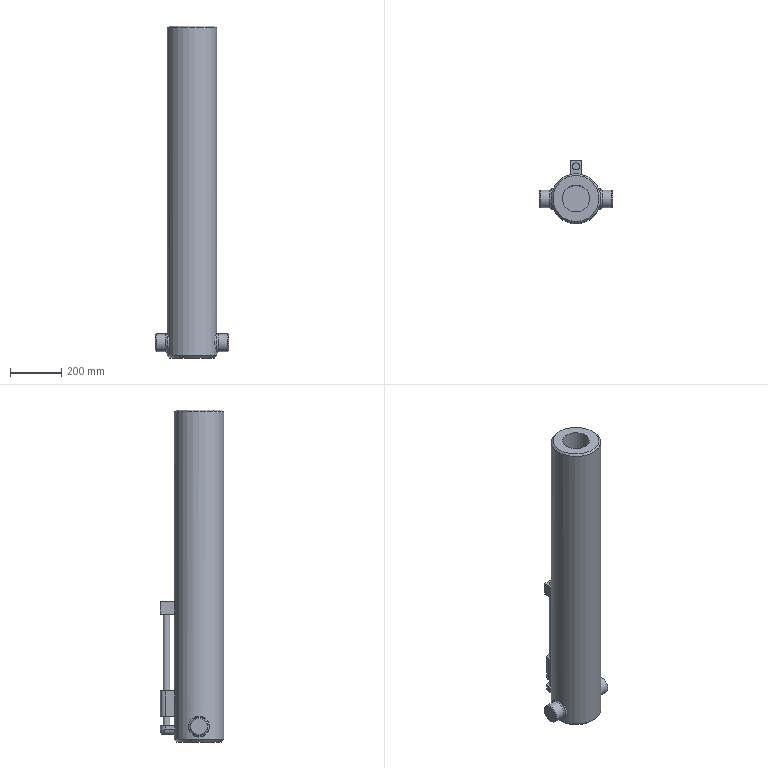Part | NX | features 推移千斤顶缸 2 | 1 solid | 49 faces | box 287 x 247.6 x 1299 mm | volume 29707096 mm3 | plane 23 | cylinder 18 | cone 4 | torus 2 | spline 2 | commonest cylinder face diameters 40 x6 81.5 x4 28.35 x2 70 x2 20 x1 28 x1
STEP:
#1=CARTESIAN_POINT('',(97.,0.,1292.4));
#2=VERTEX_POINT('',#1);
#3=CARTESIAN_POINT('',(0.,0.,1292.4));
#4=DIRECTION('',(0.,0.,1.));
#5=DIRECTION('',(1.,0.,0.));
#6=AXIS2_PLACEMENT_3D('',#3,#4,#5);
#7=CIRCLE('',#6,97.);
#8=EDGE_CURVE('',#2,#2,#7,.F.);
#9=ORIENTED_EDGE('',*,*,#8,.T.);
#10=EDGE_LOOP('',(#9));
#11=FACE_BOUND('',#10,.T.);
#12=CARTESIAN_POINT('',(-22.,94.472,65.));
#13=VERTEX_POINT('',#12);
#14=CARTESIAN_POINT('',(22.,94.472,65.));
#15=VERTEX_POINT('',#14);
#16=CARTESIAN_POINT('',(0.,0.,65.));
#17=DIRECTION('',(0.,0.,-1.));
#18=DIRECTION('',(-1.,0.,0.));
#19=AXIS2_PLACEMENT_3D('',#16,#17,#18);
#20=CIRCLE('',#19,97.);
#21=EDGE_CURVE('',#13,#15,#20,.T.);
#22=ORIENTED_EDGE('',*,*,#21,.F.);
#23=CARTESIAN_POINT('',(-22.,94.472,50.));
#24=VERTEX_POINT('',#23);
#25=CARTESIAN_POINT('',(-22.,94.472,1299.4));
#26=DIRECTION('',(0.,0.,-1.));
#27=VECTOR('',#26,1000.);
#28=LINE('',#25,#27);
#29=EDGE_CURVE('',#13,#24,#28,.T.);
#30=ORIENTED_EDGE('',*,*,#29,.T.);
#31=CARTESIAN_POINT('',(-2.,96.979,30.));
#32=VERTEX_POINT('',#31);
#33=CARTESIAN_POINT('',(-22.,94.472,50.));
#34=CARTESIAN_POINT('',(-22.,94.472,47.348));
#35=CARTESIAN_POINT('',(-20.947,94.727,42.13));
#36=CARTESIAN_POINT('',(-16.505,95.642,35.49));
#37=CARTESIAN_POINT('',(-9.89,96.59,31.062));
#38=CARTESIAN_POINT('',(-4.651,96.925,30.));
#39=CARTESIAN_POINT('',(-2.,96.979,30.));
#40=B_SPLINE_CURVE_WITH_KNOTS('',3,(#33,#34,#35,#36,#37,#38,#39),.UNSPECIFIED.,.F.,.F.,(4,1,1,1,4),(0.,0.00784,0.01568,0.02352,0.03136),.UNSPECIFIED.);
#41=EDGE_CURVE('',#24,#32,#40,.T.);
#42=ORIENTED_EDGE('',*,*,#41,.T.);
#43=CARTESIAN_POINT('',(2.,96.979,30.));
#44=VERTEX_POINT('',#43);
#45=CARTESIAN_POINT('',(0.,0.,30.));
#46=DIRECTION('',(0.,0.,-1.));
#47=DIRECTION('',(-1.,0.,0.));
#48=AXIS2_PLACEMENT_3D('',#45,#46,#47);
#49=CIRCLE('',#48,97.);
#50=EDGE_CURVE('',#32,#44,#49,.T.);
#51=ORIENTED_EDGE('',*,*,#50,.T.);
#52=CARTESIAN_POINT('',(22.,94.472,50.));
#53=VERTEX_POINT('',#52);
#54=CARTESIAN_POINT('',(2.,96.979,30.));
#55=CARTESIAN_POINT('',(4.651,96.925,30.));
#56=CARTESIAN_POINT('',(9.864,96.592,31.052));
#57=CARTESIAN_POINT('',(16.502,95.643,35.487));
#58=CARTESIAN_POINT('',(20.937,94.729,42.104));
#59=CARTESIAN_POINT('',(22.,94.472,47.348));
#60=CARTESIAN_POINT('',(22.,94.472,50.));
#61=B_SPLINE_CURVE_WITH_KNOTS('',3,(#54,#55,#56,#57,#58,#59,#60),.UNSPECIFIED.,.F.,.F.,(4,1,1,1,4),(0.,0.00784,0.01568,0.02352,0.03136),.UNSPECIFIED.);
#62=EDGE_CURVE('',#44,#53,#61,.T.);
#63=ORIENTED_EDGE('',*,*,#62,.T.);
#64=CARTESIAN_POINT('',(22.,94.472,1299.4));
#65=DIRECTION('',(0.,0.,-1.));
#66=VECTOR('',#65,1000.);
#67=LINE('',#64,#66);
#68=EDGE_CURVE('',#53,#15,#67,.F.);
#69=ORIENTED_EDGE('',*,*,#68,.T.);
#70=EDGE_LOOP('',(#22,#30,#42,#51,#63,#69));
#71=FACE_BOUND('',#70,.T.);
#72=CARTESIAN_POINT('',(97.,0.,10.));
#73=VERTEX_POINT('',#72);
#74=CARTESIAN_POINT('',(0.,0.,10.));
#75=DIRECTION('',(0.,0.,1.));
#76=DIRECTION('',(1.,0.,0.));
#77=AXIS2_PLACEMENT_3D('',#74,#75,#76);
#78=CIRCLE('',#77,97.);
#79=EDGE_CURVE('',#73,#73,#78,.T.);
#80=ORIENTED_EDGE('',*,*,#79,.T.);
#81=EDGE_LOOP('',(#80));
#82=FACE_BOUND('',#81,.T.);
#83=CARTESIAN_POINT('',(-97.,0.,100.98));
#84=VERTEX_POINT('',#83);
#85=CARTESIAN_POINT('',(-97.,0.,19.48));
#86=VERTEX_POINT('',#85);
#87=CARTESIAN_POINT('',(-97.,0.,100.98));
#88=CARTESIAN_POINT('',(-97.,2.727,100.98));
#89=CARTESIAN_POINT('',(-96.773,8.067,100.445));
#90=CARTESIAN_POINT('',(-95.472,18.439,97.265));
#91=CARTESIAN_POINT('',(-93.209,27.331,91.259));
#92=CARTESIAN_POINT('',(-90.862,34.067,83.053));
#93=CARTESIAN_POINT('',(-89.338,37.833,76.063));
#94=CARTESIAN_POINT('',(-88.276,40.215,68.295));
#95=CARTESIAN_POINT('',(-87.899,41.018,60.28));
#96=CARTESIAN_POINT('',(-88.278,40.211,52.125));
#97=CARTESIAN_POINT('',(-89.687,37.054,41.849));
#98=CARTESIAN_POINT('',(-92.06,31.015,32.891));
#99=CARTESIAN_POINT('',(-94.346,22.876,26.196));
#100=CARTESIAN_POINT('',(-95.804,15.793,22.379));
#101=CARTESIAN_POINT('',(-96.771,8.106,20.022));
#102=CARTESIAN_POINT('',(-97.,2.686,19.48));
#103=CARTESIAN_POINT('',(-97.,0.,19.48));
#104=B_SPLINE_CURVE_WITH_KNOTS('',3,(#87,#88,#89,#90,#91,#92,#93,#94,#95,#96,#97,#98,#99,#100,#101,#102,#103),.UNSPECIFIED.,.F.,.F.,(4,1,1,1,1,1,1,1,1,1,1,1,1,1,4),(0.,0.008057,0.01611,0.03223,0.04029,0.04834,0.0564,0.06446,0.07252,0.08057,0.09669,0.1047,0.1128,0.1209,0.1289),.UNSPECIFIED.);
#105=EDGE_CURVE('',#84,#86,#104,.T.);
#106=ORIENTED_EDGE('',*,*,#105,.F.);
#107=CARTESIAN_POINT('',(-97.,0.,19.48));
#108=CARTESIAN_POINT('',(-97.,-2.684,19.48));
#109=CARTESIAN_POINT('',(-96.769,-8.129,20.026));
#110=CARTESIAN_POINT('',(-95.481,-18.371,23.172));
#111=CARTESIAN_POINT('',(-93.2,-27.363,29.236));
#112=CARTESIAN_POINT('',(-90.87,-34.042,37.366));
#113=CARTESIAN_POINT('',(-89.329,-37.856,44.456));
#114=CARTESIAN_POINT('',(-88.284,-40.198,52.081));
#115=CARTESIAN_POINT('',(-87.898,-41.022,60.233));
#116=CARTESIAN_POINT('',(-88.276,-40.214,68.297));
#117=CARTESIAN_POINT('',(-89.33,-37.854,76.02));
#118=CARTESIAN_POINT('',(-90.871,-34.042,83.093));
#119=CARTESIAN_POINT('',(-93.204,-27.344,91.241));
#120=CARTESIAN_POINT('',(-96.05,-16.153,98.79));
#121=CARTESIAN_POINT('',(-97.,-5.449,100.98));
#122=CARTESIAN_POINT('',(-97.,0.,100.98));
#123=B_SPLINE_CURVE_WITH_KNOTS('',3,(#107,#108,#109,#110,#111,#112,#113,#114,#115,#116,#117,#118,#119,#120,#121,#122),.UNSPECIFIED.,.F.,.F.,(4,1,1,1,1,1,1,1,1,1,1,1,1,4),(0.1289,0.137,0.145,0.1611,0.1692,0.1772,0.1853,0.1933,0.2014,0.2094,0.2175,0.2255,0.2416,0.2577),.UNSPECIFIED.);
#124=EDGE_CURVE('',#86,#84,#123,.T.);
#125=ORIENTED_EDGE('',*,*,#124,.F.);
#126=EDGE_LOOP('',(#106,#125));
#127=FACE_BOUND('',#126,.T.);
#128=CARTESIAN_POINT('',(97.,0.,100.98));
#129=VERTEX_POINT('',#128);
#130=CARTESIAN_POINT('',(97.,0.,19.48));
#131=VERTEX_POINT('',#130);
#132=CARTESIAN_POINT('',(97.,0.,100.98));
#133=CARTESIAN_POINT('',(97.,-2.727,100.98));
#134=CARTESIAN_POINT('',(96.773,-8.067,100.445));
#135=CARTESIAN_POINT('',(95.472,-18.439,97.265));
#136=CARTESIAN_POINT('',(93.209,-27.331,91.259));
#137=CARTESIAN_POINT('',(90.862,-34.067,83.053));
#138=CARTESIAN_POINT('',(89.338,-37.833,76.063));
#139=CARTESIAN_POINT('',(88.276,-40.215,68.295));
#140=CARTESIAN_POINT('',(87.899,-41.018,60.28));
#141=CARTESIAN_POINT('',(88.278,-40.211,52.125));
#142=CARTESIAN_POINT('',(89.687,-37.054,41.849));
#143=CARTESIAN_POINT('',(92.06,-31.015,32.891));
#144=CARTESIAN_POINT('',(94.346,-22.876,26.196));
#145=CARTESIAN_POINT('',(95.804,-15.793,22.379));
#146=CARTESIAN_POINT('',(96.771,-8.106,20.022));
#147=CARTESIAN_POINT('',(97.,-2.686,19.48));
#148=CARTESIAN_POINT('',(97.,0.,19.48));
#149=B_SPLINE_CURVE_WITH_KNOTS('',3,(#132,#133,#134,#135,#136,#137,#138,#139,#140,#141,#142,#143,#144,#145,#146,#147,#148),.UNSPECIFIED.,.F.,.F.,(4,1,1,1,1,1,1,1,1,1,1,1,1,1,4),(0.,0.008057,0.01611,0.03223,0.04029,0.04834,0.0564,0.06446,0.07252,0.08057,0.09669,0.1047,0.1128,0.1209,0.1289),.UNSPECIFIED.);
#150=EDGE_CURVE('',#129,#131,#149,.T.);
#151=ORIENTED_EDGE('',*,*,#150,.F.);
#152=CARTESIAN_POINT('',(97.,0.,19.48));
#153=CARTESIAN_POINT('',(97.,2.684,19.48));
#154=CARTESIAN_POINT('',(96.769,8.129,20.026));
#155=CARTESIAN_POINT('',(95.481,18.371,23.172));
#156=CARTESIAN_POINT('',(93.2,27.363,29.236));
#157=CARTESIAN_POINT('',(90.87,34.042,37.366));
#158=CARTESIAN_POINT('',(89.329,37.856,44.456));
#159=CARTESIAN_POINT('',(88.284,40.198,52.081));
#160=CARTESIAN_POINT('',(87.898,41.022,60.233));
#161=CARTESIAN_POINT('',(88.276,40.214,68.297));
#162=CARTESIAN_POINT('',(89.33,37.854,76.02));
#163=CARTESIAN_POINT('',(90.871,34.042,83.093));
#164=CARTESIAN_POINT('',(93.204,27.344,91.241));
#165=CARTESIAN_POINT('',(96.05,16.153,98.79));
#166=CARTESIAN_POINT('',(97.,5.449,100.98));
#167=CARTESIAN_POINT('',(97.,0.,100.98));
#168=B_SPLINE_CURVE_WITH_KNOTS('',3,(#152,#153,#154,#155,#156,#157,#158,#159,#160,#161,#162,#163,#164,#165,#166,#167),.UNSPECIFIED.,.F.,.F.,(4,1,1,1,1,1,1,1,1,1,1,1,1,4),(0.1289,0.137,0.145,0.1611,0.1692,0.1772,0.1853,0.1933,0.2014,0.2094,0.2175,0.2255,0.2416,0.2577),.UNSPECIFIED.);
#169=EDGE_CURVE('',#131,#129,#168,.T.);
#170=ORIENTED_EDGE('',*,*,#169,.F.);
#171=EDGE_LOOP('',(#151,#170));
#172=FACE_BOUND('',#171,.T.);
#173=CARTESIAN_POINT('',(22.,94.472,200.));
#174=VERTEX_POINT('',#173);
#175=CARTESIAN_POINT('',(22.,94.472,100.));
#176=VERTEX_POINT('',#175);
#177=CARTESIAN_POINT('',(22.,94.472,200.));
#178=DIRECTION('',(0.,0.,-1.));
#179=VECTOR('',#178,1000.);
#180=LINE('',#177,#179);
#181=EDGE_CURVE('',#174,#176,#180,.T.);
#182=ORIENTED_EDGE('',*,*,#181,.F.);
#183=CARTESIAN_POINT('',(-22.,94.472,200.));
#184=VERTEX_POINT('',#183);
#185=CARTESIAN_POINT('',(0.,0.,200.));
#186=DIRECTION('',(0.,0.,1.));
#187=DIRECTION('',(1.,0.,0.));
#188=AXIS2_PLACEMENT_3D('',#185,#186,#187);
#189=CIRCLE('',#188,97.);
#190=EDGE_CURVE('',#174,#184,#189,.T.);
#191=ORIENTED_EDGE('',*,*,#190,.T.);
#192=CARTESIAN_POINT('',(-22.,94.472,100.));
#193=VERTEX_POINT('',#192);
#194=CARTESIAN_POINT('',(-22.,94.472,200.));
#195=DIRECTION('',(0.,0.,-1.));
#196=VECTOR('',#195,1000.);
#197=LINE('',#194,#196);
#198=EDGE_CURVE('',#184,#193,#197,.T.);
#199=ORIENTED_EDGE('',*,*,#198,.T.);
#200=CARTESIAN_POINT('',(0.,0.,100.));
#201=DIRECTION('',(0.,0.,1.));
#202=DIRECTION('',(1.,0.,0.));
#203=AXIS2_PLACEMENT_3D('',#200,#201,#202);
#204=CIRCLE('',#203,97.);
#205=EDGE_CURVE('',#176,#193,#204,.T.);
#206=ORIENTED_EDGE('',*,*,#205,.F.);
#207=EDGE_LOOP('',(#182,#191,#199,#206));
#208=FACE_BOUND('',#207,.T.);
#209=CARTESIAN_POINT('',(-22.,94.472,550.));
#210=VERTEX_POINT('',#209);
#211=CARTESIAN_POINT('',(22.,94.472,550.));
#212=VERTEX_POINT('',#211);
#213=CARTESIAN_POINT('',(0.,0.,550.));
#214=DIRECTION('',(0.,0.,-1.));
#215=DIRECTION('',(-1.,0.,0.));
#216=AXIS2_PLACEMENT_3D('',#213,#214,#215);
#217=CIRCLE('',#216,97.);
#218=EDGE_CURVE('',#210,#212,#217,.T.);
#219=ORIENTED_EDGE('',*,*,#218,.F.);
#220=CARTESIAN_POINT('',(-22.,94.472,500.));
#221=VERTEX_POINT('',#220);
#222=CARTESIAN_POINT('',(-22.,94.472,550.));
#223=DIRECTION('',(0.,0.,-1.));
#224=VECTOR('',#223,1000.);
#225=LINE('',#222,#224);
#226=EDGE_CURVE('',#210,#221,#225,.T.);
#227=ORIENTED_EDGE('',*,*,#226,.T.);
#228=CARTESIAN_POINT('',(22.,94.472,500.));
#229=VERTEX_POINT('',#228);
#230=CARTESIAN_POINT('',(0.,0.,500.));
#231=DIRECTION('',(0.,0.,-1.));
#232=DIRECTION('',(-1.,0.,0.));
#233=AXIS2_PLACEMENT_3D('',#230,#231,#232);
#234=CIRCLE('',#233,97.);
#235=EDGE_CURVE('',#221,#229,#234,.T.);
#236=ORIENTED_EDGE('',*,*,#235,.T.);
#237=CARTESIAN_POINT('',(22.,94.472,550.));
#238=DIRECTION('',(0.,0.,-1.));
#239=VECTOR('',#238,1000.);
#240=LINE('',#237,#239);
#241=EDGE_CURVE('',#212,#229,#240,.T.);
#242=ORIENTED_EDGE('',*,*,#241,.F.);
#243=EDGE_LOOP('',(#219,#227,#236,#242));
#244=FACE_BOUND('',#243,.T.);
#245=CARTESIAN_POINT('',(0.,0.,1299.4));
#246=DIRECTION('',(0.,0.,-1.));
#247=DIRECTION('',(-1.,0.,0.));
#248=AXIS2_PLACEMENT_3D('',#245,#246,#247);
#249=CYLINDRICAL_SURFACE('',#248,97.);
#250=ADVANCED_FACE('',(#11,#71,#82,#127,#172,#208,#244),#249,.T.);
#251=CARTESIAN_POINT('',(22.,130.6,200.));
#252=VERTEX_POINT('',#251);
#253=CARTESIAN_POINT('',(22.,150.6,200.));
#254=DIRECTION('',(0.,1.,0.));
#255=VECTOR('',#254,1000.);
#256=LINE('',#253,#255);
#257=EDGE_CURVE('',#174,#252,#256,.T.);
#258=ORIENTED_EDGE('',*,*,#257,.T.);
#259=CARTESIAN_POINT('',(2.,150.6,200.));
#260=VERTEX_POINT('',#259);
#261=CARTESIAN_POINT('',(2.,130.6,200.));
#262=DIRECTION('',(0.,0.,1.));
#263=DIRECTION('',(1.,0.,0.));
#264=AXIS2_PLACEMENT_3D('',#261,#262,#263);
#265=CIRCLE('',#264,20.);
#266=EDGE_CURVE('',#252,#260,#265,.T.);
#267=ORIENTED_EDGE('',*,*,#266,.T.);
#268=CARTESIAN_POINT('',(-2.,150.6,200.));
#269=VERTEX_POINT('',#268);
#270=CARTESIAN_POINT('',(-22.,150.6,200.));
#271=DIRECTION('',(-1.,0.,0.));
#272=VECTOR('',#271,1000.);
#273=LINE('',#270,#272);
#274=EDGE_CURVE('',#260,#269,#273,.T.);
#275=ORIENTED_EDGE('',*,*,#274,.T.);
#276=CARTESIAN_POINT('',(-22.,130.6,200.));
#277=VERTEX_POINT('',#276);
#278=CARTESIAN_POINT('',(-2.,130.6,200.));
#279=DIRECTION('',(0.,0.,1.));
#280=DIRECTION('',(1.,0.,0.));
#281=AXIS2_PLACEMENT_3D('',#278,#279,#280);
#282=CIRCLE('',#281,20.);
#283=EDGE_CURVE('',#269,#277,#282,.T.);
#284=ORIENTED_EDGE('',*,*,#283,.T.);
#285=CARTESIAN_POINT('',(-22.,150.6,200.));
#286=DIRECTION('',(0.,-1.,0.));
#287=VECTOR('',#286,1000.);
#288=LINE('',#285,#287);
#289=EDGE_CURVE('',#277,#184,#288,.T.);
#290=ORIENTED_EDGE('',*,*,#289,.T.);
#291=ORIENTED_EDGE('',*,*,#190,.F.);
#292=EDGE_LOOP('',(#258,#267,#275,#284,#290,#291));
#293=FACE_BOUND('',#292,.T.);
#294=CARTESIAN_POINT('',(14.175,127.56,200.));
#295=VERTEX_POINT('',#294);
#296=CARTESIAN_POINT('',(0.,127.56,200.));
#297=DIRECTION('',(0.,0.,1.));
#298=DIRECTION('',(1.,0.,0.));
#299=AXIS2_PLACEMENT_3D('',#296,#297,#298);
#300=CIRCLE('',#299,14.175);
#301=EDGE_CURVE('',#295,#295,#300,.T.);
#302=ORIENTED_EDGE('',*,*,#301,.F.);
#303=EDGE_LOOP('',(#302));
#304=FACE_BOUND('',#303,.T.);
#305=CARTESIAN_POINT('',(-22.,94.472,200.));
#306=DIRECTION('',(0.,0.,1.));
#307=DIRECTION('',(1.,0.,0.));
#308=AXIS2_PLACEMENT_3D('',#305,#306,#307);
#309=PLANE('',#308);
#310=ADVANCED_FACE('',(#293,#304),#309,.T.);
#311=CARTESIAN_POINT('',(22.,130.6,65.));
#312=VERTEX_POINT('',#311);
#313=CARTESIAN_POINT('',(22.,150.6,65.));
#314=DIRECTION('',(0.,-1.,0.));
#315=VECTOR('',#314,1000.);
#316=LINE('',#313,#315);
#317=EDGE_CURVE('',#312,#15,#316,.T.);
#318=ORIENTED_EDGE('',*,*,#317,.F.);
#319=CARTESIAN_POINT('',(2.,150.6,65.));
#320=VERTEX_POINT('',#319);
#321=CARTESIAN_POINT('',(2.,130.6,65.));
#322=DIRECTION('',(0.,0.,-1.));
#323=DIRECTION('',(-1.,0.,0.));
#324=AXIS2_PLACEMENT_3D('',#321,#322,#323);
#325=CIRCLE('',#324,20.);
#326=EDGE_CURVE('',#312,#320,#325,.F.);
#327=ORIENTED_EDGE('',*,*,#326,.T.);
#328=CARTESIAN_POINT('',(-2.,150.6,65.));
#329=VERTEX_POINT('',#328);
#330=CARTESIAN_POINT('',(22.,150.6,65.));
#331=DIRECTION('',(1.,0.,0.));
#332=VECTOR('',#331,1000.);
#333=LINE('',#330,#332);
#334=EDGE_CURVE('',#329,#320,#333,.T.);
#335=ORIENTED_EDGE('',*,*,#334,.F.);
#336=CARTESIAN_POINT('',(-22.,130.6,65.));
#337=VERTEX_POINT('',#336);
#338=CARTESIAN_POINT('',(-2.,130.6,65.));
#339=DIRECTION('',(0.,0.,-1.));
#340=DIRECTION('',(-1.,0.,0.));
#341=AXIS2_PLACEMENT_3D('',#338,#339,#340);
#342=CIRCLE('',#341,20.);
#343=EDGE_CURVE('',#329,#337,#342,.F.);
#344=ORIENTED_EDGE('',*,*,#343,.T.);
#345=CARTESIAN_POINT('',(-22.,150.6,65.));
#346=DIRECTION('',(0.,1.,0.));
#347=VECTOR('',#346,1000.);
#348=LINE('',#345,#347);
#349=EDGE_CURVE('',#13,#337,#348,.T.);
#350=ORIENTED_EDGE('',*,*,#349,.F.);
#351=ORIENTED_EDGE('',*,*,#21,.T.);
#352=EDGE_LOOP('',(#318,#327,#335,#344,#350,#351));
#353=FACE_BOUND('',#352,.T.);
#354=CARTESIAN_POINT('',(-14.175,127.56,65.));
#355=VERTEX_POINT('',#354);
#356=CARTESIAN_POINT('',(0.,127.56,65.));
#357=DIRECTION('',(0.,0.,-1.));
#358=DIRECTION('',(-1.,0.,0.));
#359=AXIS2_PLACEMENT_3D('',#356,#357,#358);
#360=CIRCLE('',#359,14.175);
#361=EDGE_CURVE('',#355,#355,#360,.F.);
#362=ORIENTED_EDGE('',*,*,#361,.F.);
#363=EDGE_LOOP('',(#362));
#364=FACE_BOUND('',#363,.T.);
#365=CARTESIAN_POINT('',(22.,90.6,65.));
#366=DIRECTION('',(0.,0.,-1.));
#367=DIRECTION('',(-1.,0.,0.));
#368=AXIS2_PLACEMENT_3D('',#365,#366,#367);
#369=PLANE('',#368);
#370=ADVANCED_FACE('',(#353,#364),#369,.F.);
#371=CARTESIAN_POINT('',(97.,0.,20.23));
#372=VERTEX_POINT('',#371);
#373=CARTESIAN_POINT('',(97.,0.,60.23));
#374=DIRECTION('',(1.,0.,0.));
#375=DIRECTION('',(0.,0.,-1.));
#376=AXIS2_PLACEMENT_3D('',#373,#374,#375);
#377=CIRCLE('',#376,40.);
#378=EDGE_CURVE('',#372,#372,#377,.F.);
#379=ORIENTED_EDGE('',*,*,#378,.T.);
#380=EDGE_LOOP('',(#379));
#381=FACE_BOUND('',#380,.T.);
#382=CARTESIAN_POINT('',(97.,0.,60.23));
#383=DIRECTION('',(1.,0.,0.));
#384=DIRECTION('',(0.,0.,-1.));
#385=AXIS2_PLACEMENT_3D('',#382,#383,#384);
#386=CIRCLE('',#385,40.75);
#387=EDGE_CURVE('',#129,#131,#386,.T.);
#388=ORIENTED_EDGE('',*,*,#387,.T.);
#389=CARTESIAN_POINT('',(97.,0.,60.23));
#390=DIRECTION('',(1.,0.,0.));
#391=DIRECTION('',(0.,0.,-1.));
#392=AXIS2_PLACEMENT_3D('',#389,#390,#391);
#393=CIRCLE('',#392,40.75);
#394=EDGE_CURVE('',#131,#129,#393,.T.);
#395=ORIENTED_EDGE('',*,*,#394,.T.);
#396=EDGE_LOOP('',(#388,#395));
#397=FACE_BOUND('',#396,.T.);
#398=CARTESIAN_POINT('',(97.,0.,60.23));
#399=DIRECTION('',(1.,0.,0.));
#400=DIRECTION('',(0.,0.,-1.));
#401=AXIS2_PLACEMENT_3D('',#398,#399,#400);
#402=PLANE('',#401);
#403=ADVANCED_FACE('',(#381,#397),#402,.T.);
#404=CARTESIAN_POINT('',(-97.,0.,20.23));
#405=VERTEX_POINT('',#404);
#406=CARTESIAN_POINT('',(-97.,0.,60.23));
#407=DIRECTION('',(1.,0.,0.));
#408=DIRECTION('',(0.,0.,-1.));
#409=AXIS2_PLACEMENT_3D('',#406,#407,#408);
#410=CIRCLE('',#409,40.);
#411=EDGE_CURVE('',#405,#405,#410,.T.);
#412=ORIENTED_EDGE('',*,*,#411,.T.);
#413=EDGE_LOOP('',(#412));
#414=FACE_BOUND('',#413,.T.);
#415=CARTESIAN_POINT('',(-97.,0.,60.23));
#416=DIRECTION('',(1.,0.,0.));
#417=DIRECTION('',(0.,0.,-1.));
#418=AXIS2_PLACEMENT_3D('',#415,#416,#417);
#419=CIRCLE('',#418,40.75);
#420=EDGE_CURVE('',#84,#86,#419,.T.);
#421=ORIENTED_EDGE('',*,*,#420,.F.);
#422=CARTESIAN_POINT('',(-97.,0.,60.23));
#423=DIRECTION('',(1.,0.,0.));
#424=DIRECTION('',(0.,0.,-1.));
#425=AXIS2_PLACEMENT_3D('',#422,#423,#424);
#426=CIRCLE('',#425,40.75);
#427=EDGE_CURVE('',#86,#84,#426,.T.);
#428=ORIENTED_EDGE('',*,*,#427,.F.);
#429=EDGE_LOOP('',(#421,#428));
#430=FACE_BOUND('',#429,.T.);
#431=CARTESIAN_POINT('',(-97.,0.,60.23));
#432=DIRECTION('',(1.,0.,0.));
#433=DIRECTION('',(0.,0.,-1.));
#434=AXIS2_PLACEMENT_3D('',#431,#432,#433);
#435=PLANE('',#434);
#436=ADVANCED_FACE('',(#414,#430),#435,.F.);
#437=CARTESIAN_POINT('',(90.,0.,1299.4));
#438=VERTEX_POINT('',#437);
#439=CARTESIAN_POINT('',(0.,0.,1299.4));
#440=DIRECTION('',(0.,0.,1.));
#441=DIRECTION('',(1.,0.,0.));
#442=AXIS2_PLACEMENT_3D('',#439,#440,#441);
#443=CIRCLE('',#442,90.);
#444=EDGE_CURVE('',#438,#438,#443,.T.);
#445=ORIENTED_EDGE('',*,*,#444,.T.);
#446=EDGE_LOOP('',(#445));
#447=FACE_BOUND('',#446,.T.);
#448=CARTESIAN_POINT('',(53.15,0.,1299.4));
#449=VERTEX_POINT('',#448);
#450=CARTESIAN_POINT('',(0.,0.,1299.4));
#451=DIRECTION('',(0.,0.,1.));
#452=DIRECTION('',(1.,0.,0.));
#453=AXIS2_PLACEMENT_3D('',#450,#451,#452);
#454=CIRCLE('',#453,53.15);
#455=EDGE_CURVE('',#449,#449,#454,.T.);
#456=ORIENTED_EDGE('',*,*,#455,.F.);
#457=EDGE_LOOP('',(#456));
#458=FACE_BOUND('',#457,.T.);
#459=CARTESIAN_POINT('',(0.,0.,1299.4));
#460=DIRECTION('',(0.,0.,1.));
#461=DIRECTION('',(1.,0.,0.));
#462=AXIS2_PLACEMENT_3D('',#459,#460,#461);
#463=PLANE('',#462);
#464=ADVANCED_FACE('',(#447,#458),#463,.T.);
#465=CARTESIAN_POINT('',(87.,0.,0.));
#466=VERTEX_POINT('',#465);
#467=CARTESIAN_POINT('',(0.,0.,0.));
#468=DIRECTION('',(0.,0.,1.));
#469=DIRECTION('',(1.,0.,0.));
#470=AXIS2_PLACEMENT_3D('',#467,#468,#469);
#471=CIRCLE('',#470,87.);
#472=EDGE_CURVE('',#466,#466,#471,.F.);
#473=ORIENTED_EDGE('',*,*,#472,.T.);
#474=EDGE_LOOP('',(#473));
#475=FACE_BOUND('',#474,.T.);
#476=CARTESIAN_POINT('',(0.,0.,0.));
#477=DIRECTION('',(0.,0.,1.));
#478=DIRECTION('',(1.,0.,0.));
#479=AXIS2_PLACEMENT_3D('',#476,#477,#478);
#480=PLANE('',#479);
#481=ADVANCED_FACE('',(#475),#480,.F.);
#482=ORIENTED_EDGE('',*,*,#420,.T.);
#483=ORIENTED_EDGE('',*,*,#124,.T.);
#484=EDGE_LOOP('',(#482,#483));
#485=FACE_BOUND('',#484,.T.);
#486=CARTESIAN_POINT('',(97.,0.,60.23));
#487=DIRECTION('',(-1.,0.,0.));
#488=DIRECTION('',(0.,0.,1.));
#489=AXIS2_PLACEMENT_3D('',#486,#487,#488);
#490=CYLINDRICAL_SURFACE('',#489,40.75);
#491=ADVANCED_FACE('',(#485),#490,.T.);
#492=ORIENTED_EDGE('',*,*,#427,.T.);
#493=ORIENTED_EDGE('',*,*,#105,.T.);
#494=EDGE_LOOP('',(#492,#493));
#495=FACE_BOUND('',#494,.T.);
#496=CARTESIAN_POINT('',(97.,0.,60.23));
#497=DIRECTION('',(-1.,0.,0.));
#498=DIRECTION('',(0.,0.,1.));
#499=AXIS2_PLACEMENT_3D('',#496,#497,#498);
#500=CYLINDRICAL_SURFACE('',#499,40.75);
#501=ADVANCED_FACE('',(#495),#500,.T.);
#502=ORIENTED_EDGE('',*,*,#387,.F.);
#503=ORIENTED_EDGE('',*,*,#150,.T.);
#504=EDGE_LOOP('',(#502,#503));
#505=FACE_BOUND('',#504,.T.);
#506=CARTESIAN_POINT('',(97.,0.,60.23));
#507=DIRECTION('',(-1.,0.,0.));
#508=DIRECTION('',(0.,0.,1.));
#509=AXIS2_PLACEMENT_3D('',#506,#507,#508);
#510=CYLINDRICAL_SURFACE('',#509,40.75);
#511=ADVANCED_FACE('',(#505),#510,.T.);
#512=ORIENTED_EDGE('',*,*,#394,.F.);
#513=ORIENTED_EDGE('',*,*,#169,.T.);
#514=EDGE_LOOP('',(#512,#513));
#515=FACE_BOUND('',#514,.T.);
#516=CARTESIAN_POINT('',(97.,0.,60.23));
#517=DIRECTION('',(-1.,0.,0.));
#518=DIRECTION('',(0.,0.,1.));
#519=AXIS2_PLACEMENT_3D('',#516,#517,#518);
#520=CYLINDRICAL_SURFACE('',#519,40.75);
#521=ADVANCED_FACE('',(#515),#520,.T.);
#522=CARTESIAN_POINT('',(-140.5,0.,95.23));
#523=VERTEX_POINT('',#522);
#524=CARTESIAN_POINT('',(-140.5,0.,60.23));
#525=DIRECTION('',(-1.,0.,0.));
#526=DIRECTION('',(0.,0.,1.));
#527=AXIS2_PLACEMENT_3D('',#524,#525,#526);
#528=CIRCLE('',#527,35.);
#529=EDGE_CURVE('',#523,#523,#528,.F.);
#530=ORIENTED_EDGE('',*,*,#529,.T.);
#531=EDGE_LOOP('',(#530));
#532=FACE_BOUND('',#531,.T.);
#533=CARTESIAN_POINT('',(-102.,0.,25.23));
#534=VERTEX_POINT('',#533);
#535=CARTESIAN_POINT('',(-102.,0.,60.23));
#536=DIRECTION('',(1.,0.,0.));
#537=DIRECTION('',(0.,0.,-1.));
#538=AXIS2_PLACEMENT_3D('',#535,#536,#537);
#539=CIRCLE('',#538,35.);
#540=EDGE_CURVE('',#534,#534,#539,.F.);
#541=ORIENTED_EDGE('',*,*,#540,.T.);
#542=EDGE_LOOP('',(#541));
#543=FACE_BOUND('',#542,.T.);
#544=CARTESIAN_POINT('',(-143.5,0.,60.23));
#545=DIRECTION('',(1.,0.,0.));
#546=DIRECTION('',(0.,0.,-1.));
#547=AXIS2_PLACEMENT_3D('',#544,#545,#546);
#548=CYLINDRICAL_SURFACE('',#547,35.);
#549=ADVANCED_FACE('',(#532,#543),#548,.T.);
#550=CARTESIAN_POINT('',(-143.5,0.,92.23));
#551=VERTEX_POINT('',#550);
#552=CARTESIAN_POINT('',(-143.5,0.,60.23));
#553=DIRECTION('',(-1.,0.,0.));
#554=DIRECTION('',(0.,0.,1.));
#555=AXIS2_PLACEMENT_3D('',#552,#553,#554);
#556=CIRCLE('',#555,32.);
#557=EDGE_CURVE('',#551,#551,#556,.T.);
#558=ORIENTED_EDGE('',*,*,#557,.T.);
#559=EDGE_LOOP('',(#558));
#560=FACE_BOUND('',#559,.T.);
#561=CARTESIAN_POINT('',(-143.5,0.,60.23));
#562=DIRECTION('',(-1.,0.,0.));
#563=DIRECTION('',(0.,0.,1.));
#564=AXIS2_PLACEMENT_3D('',#561,#562,#563);
#565=PLANE('',#564);
#566=ADVANCED_FACE('',(#560),#565,.T.);
#567=CARTESIAN_POINT('',(140.5,0.,25.23));
#568=VERTEX_POINT('',#567);
#569=CARTESIAN_POINT('',(140.5,0.,60.23));
#570=DIRECTION('',(1.,0.,0.));
#571=DIRECTION('',(0.,0.,-1.));
#572=AXIS2_PLACEMENT_3D('',#569,#570,#571);
#573=CIRCLE('',#572,35.);
#574=EDGE_CURVE('',#568,#568,#573,.F.);
#575=ORIENTED_EDGE('',*,*,#574,.T.);
#576=EDGE_LOOP('',(#575));
#577=FACE_BOUND('',#576,.T.);
#578=CARTESIAN_POINT('',(102.,0.,25.23));
#579=VERTEX_POINT('',#578);
#580=CARTESIAN_POINT('',(102.,0.,60.23));
#581=DIRECTION('',(1.,0.,0.));
#582=DIRECTION('',(0.,0.,-1.));
#583=AXIS2_PLACEMENT_3D('',#580,#581,#582);
#584=CIRCLE('',#583,35.);
#585=EDGE_CURVE('',#579,#579,#584,.T.);
#586=ORIENTED_EDGE('',*,*,#585,.T.);
#587=EDGE_LOOP('',(#586));
#588=FACE_BOUND('',#587,.T.);
#589=CARTESIAN_POINT('',(143.5,0.,60.23));
#590=DIRECTION('',(-1.,0.,0.));
#591=DIRECTION('',(0.,0.,1.));
#592=AXIS2_PLACEMENT_3D('',#589,#590,#591);
#593=CYLINDRICAL_SURFACE('',#592,35.);
#594=ADVANCED_FACE('',(#577,#588),#593,.T.);
#595=CARTESIAN_POINT('',(143.5,0.,28.23));
#596=VERTEX_POINT('',#595);
#597=CARTESIAN_POINT('',(143.5,0.,60.23));
#598=DIRECTION('',(1.,0.,0.));
#599=DIRECTION('',(0.,0.,-1.));
#600=AXIS2_PLACEMENT_3D('',#597,#598,#599);
#601=CIRCLE('',#600,32.);
#602=EDGE_CURVE('',#596,#596,#601,.T.);
#603=ORIENTED_EDGE('',*,*,#602,.T.);
#604=EDGE_LOOP('',(#603));
#605=FACE_BOUND('',#604,.T.);
#606=CARTESIAN_POINT('',(143.5,0.,60.23));
#607=DIRECTION('',(1.,0.,0.));
#608=DIRECTION('',(0.,0.,-1.));
#609=AXIS2_PLACEMENT_3D('',#606,#607,#608);
#610=PLANE('',#609);
#611=ADVANCED_FACE('',(#605),#610,.T.);
#612=ORIENTED_EDGE('',*,*,#378,.F.);
#613=EDGE_LOOP('',(#612));
#614=FACE_BOUND('',#613,.T.);
#615=ORIENTED_EDGE('',*,*,#585,.F.);
#616=EDGE_LOOP('',(#615));
#617=FACE_BOUND('',#616,.T.);
#618=CARTESIAN_POINT('',(102.,0.,60.23));
#619=DIRECTION('',(1.,0.,0.));
#620=DIRECTION('',(0.,0.,-1.));
#621=AXIS2_PLACEMENT_3D('',#618,#619,#620);
#622=TOROIDAL_SURFACE('',#621,40.,5.);
#623=ADVANCED_FACE('',(#614,#617),#622,.F.);
#624=ORIENTED_EDGE('',*,*,#411,.F.);
#625=EDGE_LOOP('',(#624));
#626=FACE_BOUND('',#625,.T.);
#627=ORIENTED_EDGE('',*,*,#540,.F.);
#628=EDGE_LOOP('',(#627));
#629=FACE_BOUND('',#628,.T.);
#630=CARTESIAN_POINT('',(-102.,0.,60.23));
#631=DIRECTION('',(1.,0.,0.));
#632=DIRECTION('',(0.,0.,-1.));
#633=AXIS2_PLACEMENT_3D('',#630,#631,#632);
#634=TOROIDAL_SURFACE('',#633,40.,5.);
#635=ADVANCED_FACE('',(#626,#629),#634,.F.);
#636=ORIENTED_EDGE('',*,*,#574,.F.);
#637=EDGE_LOOP('',(#636));
#638=FACE_BOUND('',#637,.T.);
#639=ORIENTED_EDGE('',*,*,#602,.F.);
#640=EDGE_LOOP('',(#639));
#641=FACE_BOUND('',#640,.T.);
#642=CARTESIAN_POINT('',(143.5,0.,60.23));
#643=DIRECTION('',(-1.,0.,0.));
#644=DIRECTION('',(0.,0.,1.));
#645=AXIS2_PLACEMENT_3D('',#642,#643,#644);
#646=CONICAL_SURFACE('',#645,32.,0.7854);
#647=ADVANCED_FACE('',(#638,#641),#646,.T.);
#648=ORIENTED_EDGE('',*,*,#529,.F.);
#649=EDGE_LOOP('',(#648));
#650=FACE_BOUND('',#649,.T.);
#651=ORIENTED_EDGE('',*,*,#557,.F.);
#652=EDGE_LOOP('',(#651));
#653=FACE_BOUND('',#652,.T.);
#654=CARTESIAN_POINT('',(-143.5,0.,60.23));
#655=DIRECTION('',(1.,0.,0.));
#656=DIRECTION('',(0.,0.,-1.));
#657=AXIS2_PLACEMENT_3D('',#654,#655,#656);
#658=CONICAL_SURFACE('',#657,32.,0.7854);
#659=ADVANCED_FACE('',(#650,#653),#658,.T.);
#660=ORIENTED_EDGE('',*,*,#472,.F.);
#661=EDGE_LOOP('',(#660));
#662=FACE_BOUND('',#661,.T.);
#663=ORIENTED_EDGE('',*,*,#79,.F.);
#664=EDGE_LOOP('',(#663));
#665=FACE_BOUND('',#664,.T.);
#666=CARTESIAN_POINT('',(0.,0.,10.));
#667=DIRECTION('',(0.,0.,1.));
#668=DIRECTION('',(1.,0.,0.));
#669=AXIS2_PLACEMENT_3D('',#666,#667,#668);
#670=CONICAL_SURFACE('',#669,97.,0.7854);
#671=ADVANCED_FACE('',(#662,#665),#670,.T.);
#672=CARTESIAN_POINT('',(53.15,0.,212.74));
#673=VERTEX_POINT('',#672);
#674=CARTESIAN_POINT('',(0.,0.,212.74));
#675=DIRECTION('',(0.,0.,1.));
#676=DIRECTION('',(1.,0.,0.));
#677=AXIS2_PLACEMENT_3D('',#674,#675,#676);
#678=CIRCLE('',#677,53.15);
#679=EDGE_CURVE('',#673,#673,#678,.T.);
#680=ORIENTED_EDGE('',*,*,#679,.F.);
#681=EDGE_LOOP('',(#680));
#682=FACE_BOUND('',#681,.T.);
#683=ORIENTED_EDGE('',*,*,#455,.T.);
#684=EDGE_LOOP('',(#683));
#685=FACE_BOUND('',#684,.T.);
#686=CARTESIAN_POINT('',(0.,0.,212.74));
#687=DIRECTION('',(0.,0.,1.));
#688=DIRECTION('',(1.,0.,0.));
#689=AXIS2_PLACEMENT_3D('',#686,#687,#688);
#690=CYLINDRICAL_SURFACE('',#689,53.15);
#691=ADVANCED_FACE('',(#682,#685),#690,.F.);
#692=ORIENTED_EDGE('',*,*,#679,.T.);
#693=EDGE_LOOP('',(#692));
#694=FACE_BOUND('',#693,.T.);
#695=CARTESIAN_POINT('',(0.,0.,212.74));
#696=DIRECTION('',(0.,0.,1.));
#697=DIRECTION('',(1.,0.,0.));
#698=AXIS2_PLACEMENT_3D('',#695,#696,#697);
#699=PLANE('',#698);
#700=ADVANCED_FACE('',(#694),#699,.T.);
#701=ORIENTED_EDGE('',*,*,#68,.F.);
#702=CARTESIAN_POINT('',(22.,130.6,50.));
#703=VERTEX_POINT('',#702);
#704=CARTESIAN_POINT('',(22.,150.6,50.));
#705=DIRECTION('',(0.,-1.,0.));
#706=VECTOR('',#705,1000.);
#707=LINE('',#704,#706);
#708=EDGE_CURVE('',#53,#703,#707,.F.);
#709=ORIENTED_EDGE('',*,*,#708,.T.);
#710=CARTESIAN_POINT('',(22.,130.6,65.));
#711=DIRECTION('',(0.,0.,-1.));
#712=VECTOR('',#711,1000.);
#713=LINE('',#710,#712);
#714=EDGE_CURVE('',#703,#312,#713,.F.);
#715=ORIENTED_EDGE('',*,*,#714,.T.);
#716=ORIENTED_EDGE('',*,*,#317,.T.);
#717=EDGE_LOOP('',(#701,#709,#715,#716));
#718=FACE_BOUND('',#717,.T.);
#719=CARTESIAN_POINT('',(22.,150.6,65.));
#720=DIRECTION('',(1.,0.,0.));
#721=DIRECTION('',(0.,1.,0.));
#722=AXIS2_PLACEMENT_3D('',#719,#720,#721);
#723=PLANE('',#722);
#724=ADVANCED_FACE('',(#718),#723,.T.);
#725=CARTESIAN_POINT('',(-22.,130.6,50.));
#726=VERTEX_POINT('',#725);
#727=CARTESIAN_POINT('',(-22.,130.6,65.));
#728=DIRECTION('',(0.,0.,-1.));
#729=VECTOR('',#728,1000.);
#730=LINE('',#727,#729);
#731=EDGE_CURVE('',#337,#726,#730,.T.);
#732=ORIENTED_EDGE('',*,*,#731,.T.);
#733=CARTESIAN_POINT('',(-22.,150.6,50.));
#734=DIRECTION('',(0.,1.,0.));
#735=VECTOR('',#734,1000.);
#736=LINE('',#733,#735);
#737=EDGE_CURVE('',#726,#24,#736,.F.);
#738=ORIENTED_EDGE('',*,*,#737,.T.);
#739=ORIENTED_EDGE('',*,*,#29,.F.);
#740=ORIENTED_EDGE('',*,*,#349,.T.);
#741=EDGE_LOOP('',(#732,#738,#739,#740));
#742=FACE_BOUND('',#741,.T.);
#743=CARTESIAN_POINT('',(-22.,150.6,65.));
#744=DIRECTION('',(-1.,0.,0.));
#745=DIRECTION('',(0.,-1.,0.));
#746=AXIS2_PLACEMENT_3D('',#743,#744,#745);
#747=PLANE('',#746);
#748=ADVANCED_FACE('',(#742),#747,.T.);
#749=CARTESIAN_POINT('',(-2.,140.6,30.));
#750=VERTEX_POINT('',#749);
#751=CARTESIAN_POINT('',(2.,140.6,30.));
#752=VERTEX_POINT('',#751);
#753=CARTESIAN_POINT('',(22.,140.6,30.));
#754=DIRECTION('',(1.,0.,0.));
#755=VECTOR('',#754,1000.);
#756=LINE('',#753,#755);
#757=EDGE_CURVE('',#750,#752,#756,.T.);
#758=ORIENTED_EDGE('',*,*,#757,.T.);
#759=CARTESIAN_POINT('',(2.,90.6,30.));
#760=DIRECTION('',(0.,-1.,0.));
#761=VECTOR('',#760,1000.);
#762=LINE('',#759,#761);
#763=EDGE_CURVE('',#752,#44,#762,.T.);
#764=ORIENTED_EDGE('',*,*,#763,.T.);
#765=ORIENTED_EDGE('',*,*,#50,.F.);
#766=CARTESIAN_POINT('',(-2.,90.6,30.));
#767=DIRECTION('',(0.,1.,0.));
#768=VECTOR('',#767,1000.);
#769=LINE('',#766,#768);
#770=EDGE_CURVE('',#32,#750,#769,.T.);
#771=ORIENTED_EDGE('',*,*,#770,.T.);
#772=EDGE_LOOP('',(#758,#764,#765,#771));
#773=FACE_BOUND('',#772,.T.);
#774=CARTESIAN_POINT('',(22.,90.6,30.));
#775=DIRECTION('',(0.,0.,-1.));
#776=DIRECTION('',(-1.,0.,0.));
#777=AXIS2_PLACEMENT_3D('',#774,#775,#776);
#778=PLANE('',#777);
#779=ADVANCED_FACE('',(#773),#778,.T.);
#780=ORIENTED_EDGE('',*,*,#334,.T.);
#781=CARTESIAN_POINT('',(2.,150.6,40.));
#782=VERTEX_POINT('',#781);
#783=CARTESIAN_POINT('',(2.,150.6,65.));
#784=DIRECTION('',(0.,0.,-1.));
#785=VECTOR('',#784,1000.);
#786=LINE('',#783,#785);
#787=EDGE_CURVE('',#320,#782,#786,.T.);
#788=ORIENTED_EDGE('',*,*,#787,.T.);
#789=CARTESIAN_POINT('',(-2.,150.6,40.));
#790=VERTEX_POINT('',#789);
#791=CARTESIAN_POINT('',(22.,150.6,40.));
#792=DIRECTION('',(1.,0.,0.));
#793=VECTOR('',#792,1000.);
#794=LINE('',#791,#793);
#795=EDGE_CURVE('',#782,#790,#794,.F.);
#796=ORIENTED_EDGE('',*,*,#795,.T.);
#797=CARTESIAN_POINT('',(-2.,150.6,65.));
#798=DIRECTION('',(0.,0.,-1.));
#799=VECTOR('',#798,1000.);
#800=LINE('',#797,#799);
#801=EDGE_CURVE('',#790,#329,#800,.F.);
#802=ORIENTED_EDGE('',*,*,#801,.T.);
#803=EDGE_LOOP('',(#780,#788,#796,#802));
#804=FACE_BOUND('',#803,.T.);
#805=CARTESIAN_POINT('',(22.,150.6,65.));
#806=DIRECTION('',(0.,1.,0.));
#807=DIRECTION('',(0.,0.,1.));
#808=AXIS2_PLACEMENT_3D('',#805,#806,#807);
#809=PLANE('',#808);
#810=ADVANCED_FACE('',(#804),#809,.T.);
#811=CARTESIAN_POINT('',(14.175,127.56,100.));
#812=VERTEX_POINT('',#811);
#813=CARTESIAN_POINT('',(0.,127.56,100.));
#814=DIRECTION('',(0.,0.,1.));
#815=DIRECTION('',(1.,0.,0.));
#816=AXIS2_PLACEMENT_3D('',#813,#814,#815);
#817=CIRCLE('',#816,14.175);
#818=EDGE_CURVE('',#812,#812,#817,.T.);
#819=ORIENTED_EDGE('',*,*,#818,.F.);
#820=EDGE_LOOP('',(#819));
#821=FACE_BOUND('',#820,.T.);
#822=ORIENTED_EDGE('',*,*,#361,.T.);
#823=EDGE_LOOP('',(#822));
#824=FACE_BOUND('',#823,.T.);
#825=CARTESIAN_POINT('',(0.,127.56,100.));
#826=DIRECTION('',(0.,0.,-1.));
#827=DIRECTION('',(-1.,0.,0.));
#828=AXIS2_PLACEMENT_3D('',#825,#826,#827);
#829=CYLINDRICAL_SURFACE('',#828,14.175);
#830=ADVANCED_FACE('',(#821,#824),#829,.T.);
#831=ORIENTED_EDGE('',*,*,#818,.T.);
#832=EDGE_LOOP('',(#831));
#833=FACE_BOUND('',#832,.T.);
#834=CARTESIAN_POINT('',(2.,150.6,100.));
#835=VERTEX_POINT('',#834);
#836=CARTESIAN_POINT('',(-2.,150.6,100.));
#837=VERTEX_POINT('',#836);
#838=CARTESIAN_POINT('',(-22.,150.6,100.));
#839=DIRECTION('',(-1.,0.,0.));
#840=VECTOR('',#839,1000.);
#841=LINE('',#838,#840);
#842=EDGE_CURVE('',#835,#837,#841,.T.);
#843=ORIENTED_EDGE('',*,*,#842,.F.);
#844=CARTESIAN_POINT('',(22.,130.6,100.));
#845=VERTEX_POINT('',#844);
#846=CARTESIAN_POINT('',(2.,130.6,100.));
#847=DIRECTION('',(0.,0.,1.));
#848=DIRECTION('',(1.,0.,0.));
#849=AXIS2_PLACEMENT_3D('',#846,#847,#848);
#850=CIRCLE('',#849,20.);
#851=EDGE_CURVE('',#835,#845,#850,.F.);
#852=ORIENTED_EDGE('',*,*,#851,.T.);
#853=CARTESIAN_POINT('',(22.,150.6,100.));
#854=DIRECTION('',(0.,1.,0.));
#855=VECTOR('',#854,1000.);
#856=LINE('',#853,#855);
#857=EDGE_CURVE('',#176,#845,#856,.T.);
#858=ORIENTED_EDGE('',*,*,#857,.F.);
#859=ORIENTED_EDGE('',*,*,#205,.T.);
#860=CARTESIAN_POINT('',(-22.,130.6,100.));
#861=VERTEX_POINT('',#860);
#862=CARTESIAN_POINT('',(-22.,150.6,100.));
#863=DIRECTION('',(0.,-1.,0.));
#864=VECTOR('',#863,1000.);
#865=LINE('',#862,#864);
#866=EDGE_CURVE('',#861,#193,#865,.T.);
#867=ORIENTED_EDGE('',*,*,#866,.F.);
#868=CARTESIAN_POINT('',(-2.,130.6,100.));
#869=DIRECTION('',(0.,0.,1.));
#870=DIRECTION('',(1.,0.,0.));
#871=AXIS2_PLACEMENT_3D('',#868,#869,#870);
#872=CIRCLE('',#871,20.);
#873=EDGE_CURVE('',#861,#837,#872,.F.);
#874=ORIENTED_EDGE('',*,*,#873,.T.);
#875=EDGE_LOOP('',(#843,#852,#858,#859,#867,#874));
#876=FACE_BOUND('',#875,.T.);
#877=CARTESIAN_POINT('',(-22.,94.472,100.));
#878=DIRECTION('',(0.,0.,1.));
#879=DIRECTION('',(1.,0.,0.));
#880=AXIS2_PLACEMENT_3D('',#877,#878,#879);
#881=PLANE('',#880);
#882=ADVANCED_FACE('',(#833,#876),#881,.F.);
#883=ORIENTED_EDGE('',*,*,#289,.F.);
#884=CARTESIAN_POINT('',(-22.,130.6,200.));
#885=DIRECTION('',(0.,0.,-1.));
#886=VECTOR('',#885,1000.);
#887=LINE('',#884,#886);
#888=EDGE_CURVE('',#277,#861,#887,.T.);
#889=ORIENTED_EDGE('',*,*,#888,.T.);
#890=ORIENTED_EDGE('',*,*,#866,.T.);
#891=ORIENTED_EDGE('',*,*,#198,.F.);
#892=EDGE_LOOP('',(#883,#889,#890,#891));
#893=FACE_BOUND('',#892,.T.);
#894=CARTESIAN_POINT('',(-22.,150.6,200.));
#895=DIRECTION('',(1.,0.,0.));
#896=DIRECTION('',(0.,0.,-1.));
#897=AXIS2_PLACEMENT_3D('',#894,#895,#896);
#898=PLANE('',#897);
#899=ADVANCED_FACE('',(#893),#898,.F.);
#900=ORIENTED_EDGE('',*,*,#857,.T.);
#901=CARTESIAN_POINT('',(22.,130.6,200.));
#902=DIRECTION('',(0.,0.,-1.));
#903=VECTOR('',#902,1000.);
#904=LINE('',#901,#903);
#905=EDGE_CURVE('',#845,#252,#904,.F.);
#906=ORIENTED_EDGE('',*,*,#905,.T.);
#907=ORIENTED_EDGE('',*,*,#257,.F.);
#908=ORIENTED_EDGE('',*,*,#181,.T.);
#909=EDGE_LOOP('',(#900,#906,#907,#908));
#910=FACE_BOUND('',#909,.T.);
#911=CARTESIAN_POINT('',(22.,150.6,200.));
#912=DIRECTION('',(-1.,0.,0.));
#913=DIRECTION('',(0.,0.,1.));
#914=AXIS2_PLACEMENT_3D('',#911,#912,#913);
#915=PLANE('',#914);
#916=ADVANCED_FACE('',(#910),#915,.F.);
#917=ORIENTED_EDGE('',*,*,#274,.F.);
#918=CARTESIAN_POINT('',(2.,150.6,200.));
#919=DIRECTION('',(0.,0.,-1.));
#920=VECTOR('',#919,1000.);
#921=LINE('',#918,#920);
#922=EDGE_CURVE('',#260,#835,#921,.T.);
#923=ORIENTED_EDGE('',*,*,#922,.T.);
#924=ORIENTED_EDGE('',*,*,#842,.T.);
#925=CARTESIAN_POINT('',(-2.,150.6,200.));
#926=DIRECTION('',(0.,0.,-1.));
#927=VECTOR('',#926,1000.);
#928=LINE('',#925,#927);
#929=EDGE_CURVE('',#837,#269,#928,.F.);
#930=ORIENTED_EDGE('',*,*,#929,.T.);
#931=EDGE_LOOP('',(#917,#923,#924,#930));
#932=FACE_BOUND('',#931,.T.);
#933=CARTESIAN_POINT('',(-22.,150.6,200.));
#934=DIRECTION('',(0.,-1.,0.));
#935=DIRECTION('',(0.,0.,-1.));
#936=AXIS2_PLACEMENT_3D('',#933,#934,#935);
#937=PLANE('',#936);
#938=ADVANCED_FACE('',(#932),#937,.F.);
#939=CARTESIAN_POINT('',(14.175,127.56,500.));
#940=VERTEX_POINT('',#939);
#941=CARTESIAN_POINT('',(0.,127.56,500.));
#942=DIRECTION('',(0.,0.,1.));
#943=DIRECTION('',(1.,0.,0.));
#944=AXIS2_PLACEMENT_3D('',#941,#942,#943);
#945=CIRCLE('',#944,14.175);
#946=EDGE_CURVE('',#940,#940,#945,.T.);
#947=ORIENTED_EDGE('',*,*,#946,.F.);
#948=EDGE_LOOP('',(#947));
#949=FACE_BOUND('',#948,.T.);
#950=ORIENTED_EDGE('',*,*,#301,.T.);
#951=EDGE_LOOP('',(#950));
#952=FACE_BOUND('',#951,.T.);
#953=CARTESIAN_POINT('',(0.,127.56,500.));
#954=DIRECTION('',(0.,0.,-1.));
#955=DIRECTION('',(-1.,0.,0.));
#956=AXIS2_PLACEMENT_3D('',#953,#954,#955);
#957=CYLINDRICAL_SURFACE('',#956,14.175);
#958=ADVANCED_FACE('',(#949,#952),#957,.T.);
#959=CARTESIAN_POINT('',(14.,127.,550.));
#960=VERTEX_POINT('',#959);
#961=CARTESIAN_POINT('',(0.,127.,550.));
#962=DIRECTION('',(0.,0.,1.));
#963=DIRECTION('',(1.,0.,0.));
#964=AXIS2_PLACEMENT_3D('',#961,#962,#963);
#965=CIRCLE('',#964,14.);
#966=EDGE_CURVE('',#960,#960,#965,.T.);
#967=ORIENTED_EDGE('',*,*,#966,.F.);
#968=EDGE_LOOP('',(#967));
#969=FACE_BOUND('',#968,.T.);
#970=CARTESIAN_POINT('',(-22.,150.6,550.));
#971=VERTEX_POINT('',#970);
#972=CARTESIAN_POINT('',(-22.,150.6,550.));
#973=DIRECTION('',(0.,-1.,0.));
#974=VECTOR('',#973,1000.);
#975=LINE('',#972,#974);
#976=EDGE_CURVE('',#971,#210,#975,.T.);
#977=ORIENTED_EDGE('',*,*,#976,.T.);
#978=ORIENTED_EDGE('',*,*,#218,.T.);
#979=CARTESIAN_POINT('',(22.,150.6,550.));
#980=VERTEX_POINT('',#979);
#981=CARTESIAN_POINT('',(22.,150.6,550.));
#982=DIRECTION('',(0.,1.,0.));
#983=VECTOR('',#982,1000.);
#984=LINE('',#981,#983);
#985=EDGE_CURVE('',#212,#980,#984,.T.);
#986=ORIENTED_EDGE('',*,*,#985,.T.);
#987=CARTESIAN_POINT('',(22.,150.6,550.));
#988=DIRECTION('',(-1.,0.,0.));
#989=VECTOR('',#988,1000.);
#990=LINE('',#987,#989);
#991=EDGE_CURVE('',#980,#971,#990,.T.);
#992=ORIENTED_EDGE('',*,*,#991,.T.);
#993=EDGE_LOOP('',(#977,#978,#986,#992));
#994=FACE_BOUND('',#993,.T.);
#995=CARTESIAN_POINT('',(22.,94.472,550.));
#996=DIRECTION('',(0.,0.,-1.));
#997=DIRECTION('',(-1.,0.,0.));
#998=AXIS2_PLACEMENT_3D('',#995,#996,#997);
#999=PLANE('',#998);
#1000=ADVANCED_FACE('',(#969,#994),#999,.F.);
#1001=ORIENTED_EDGE('',*,*,#946,.T.);
#1002=EDGE_LOOP('',(#1001));
#1003=FACE_BOUND('',#1002,.T.);
#1004=ORIENTED_EDGE('',*,*,#235,.F.);
#1005=CARTESIAN_POINT('',(-22.,150.6,500.));
#1006=VERTEX_POINT('',#1005);
#1007=CARTESIAN_POINT('',(-22.,150.6,500.));
#1008=DIRECTION('',(0.,-1.,0.));
#1009=VECTOR('',#1008,1000.);
#1010=LINE('',#1007,#1009);
#1011=EDGE_CURVE('',#1006,#221,#1010,.T.);
#1012=ORIENTED_EDGE('',*,*,#1011,.F.);
#1013=CARTESIAN_POINT('',(22.,150.6,500.));
#1014=VERTEX_POINT('',#1013);
#1015=CARTESIAN_POINT('',(22.,150.6,500.));
#1016=DIRECTION('',(-1.,0.,0.));
#1017=VECTOR('',#1016,1000.);
#1018=LINE('',#1015,#1017);
#1019=EDGE_CURVE('',#1014,#1006,#1018,.T.);
#1020=ORIENTED_EDGE('',*,*,#1019,.F.);
#1021=CARTESIAN_POINT('',(22.,150.6,500.));
#1022=DIRECTION('',(0.,1.,0.));
#1023=VECTOR('',#1022,1000.);
#1024=LINE('',#1021,#1023);
#1025=EDGE_CURVE('',#229,#1014,#1024,.T.);
#1026=ORIENTED_EDGE('',*,*,#1025,.F.);
#1027=EDGE_LOOP('',(#1004,#1012,#1020,#1026));
#1028=FACE_BOUND('',#1027,.T.);
#1029=CARTESIAN_POINT('',(22.,94.472,500.));
#1030=DIRECTION('',(0.,0.,-1.));
#1031=DIRECTION('',(-1.,0.,0.));
#1032=AXIS2_PLACEMENT_3D('',#1029,#1030,#1031);
#1033=PLANE('',#1032);
#1034=ADVANCED_FACE('',(#1003,#1028),#1033,.T.);
#1035=ORIENTED_EDGE('',*,*,#1025,.T.);
#1036=CARTESIAN_POINT('',(22.,150.6,550.));
#1037=DIRECTION('',(0.,0.,-1.));
#1038=VECTOR('',#1037,1000.);
#1039=LINE('',#1036,#1038);
#1040=EDGE_CURVE('',#980,#1014,#1039,.T.);
#1041=ORIENTED_EDGE('',*,*,#1040,.F.);
#1042=ORIENTED_EDGE('',*,*,#985,.F.);
#1043=ORIENTED_EDGE('',*,*,#241,.T.);
#1044=EDGE_LOOP('',(#1035,#1041,#1042,#1043));
#1045=FACE_BOUND('',#1044,.T.);
#1046=CARTESIAN_POINT('',(22.,150.6,550.));
#1047=DIRECTION('',(-1.,0.,0.));
#1048=DIRECTION('',(0.,0.,1.));
#1049=AXIS2_PLACEMENT_3D('',#1046,#1047,#1048);
#1050=PLANE('',#1049);
#1051=ADVANCED_FACE('',(#1045),#1050,.F.);
#1052=ORIENTED_EDGE('',*,*,#1019,.T.);
#1053=CARTESIAN_POINT('',(-22.,150.6,550.));
#1054=DIRECTION('',(0.,0.,-1.));
#1055=VECTOR('',#1054,1000.);
#1056=LINE('',#1053,#1055);
#1057=EDGE_CURVE('',#971,#1006,#1056,.T.);
#1058=ORIENTED_EDGE('',*,*,#1057,.F.);
#1059=ORIENTED_EDGE('',*,*,#991,.F.);
#1060=ORIENTED_EDGE('',*,*,#1040,.T.);
#1061=EDGE_LOOP('',(#1052,#1058,#1059,#1060));
#1062=FACE_BOUND('',#1061,.T.);
#1063=CARTESIAN_POINT('',(22.,150.6,550.));
#1064=DIRECTION('',(0.,-1.,0.));
#1065=DIRECTION('',(0.,0.,-1.));
#1066=AXIS2_PLACEMENT_3D('',#1063,#1064,#1065);
#1067=PLANE('',#1066);
#1068=ADVANCED_FACE('',(#1062),#1067,.F.);
#1069=ORIENTED_EDGE('',*,*,#1011,.T.);
#1070=ORIENTED_EDGE('',*,*,#226,.F.);
#1071=ORIENTED_EDGE('',*,*,#976,.F.);
#1072=ORIENTED_EDGE('',*,*,#1057,.T.);
#1073=EDGE_LOOP('',(#1069,#1070,#1071,#1072));
#1074=FACE_BOUND('',#1073,.T.);
#1075=CARTESIAN_POINT('',(-22.,150.6,550.));
#1076=DIRECTION('',(1.,0.,0.));
#1077=DIRECTION('',(0.,0.,-1.));
#1078=AXIS2_PLACEMENT_3D('',#1075,#1076,#1077);
#1079=PLANE('',#1078);
#1080=ADVANCED_FACE('',(#1074),#1079,.F.);
#1081=ORIENTED_EDGE('',*,*,#8,.F.);
#1082=EDGE_LOOP('',(#1081));
#1083=FACE_BOUND('',#1082,.T.);
#1084=ORIENTED_EDGE('',*,*,#444,.F.);
#1085=EDGE_LOOP('',(#1084));
#1086=FACE_BOUND('',#1085,.T.);
#1087=CARTESIAN_POINT('',(0.,0.,1299.4));
#1088=DIRECTION('',(0.,0.,-1.));
#1089=DIRECTION('',(-1.,0.,0.));
#1090=AXIS2_PLACEMENT_3D('',#1087,#1088,#1089);
#1091=CONICAL_SURFACE('',#1090,90.,0.7854);
#1092=ADVANCED_FACE('',(#1083,#1086),#1091,.T.);
#1093=ORIENTED_EDGE('',*,*,#795,.F.);
#1094=CARTESIAN_POINT('',(2.,140.6,40.));
#1095=DIRECTION('',(-1.,0.,0.));
#1096=DIRECTION('',(0.,0.,1.));
#1097=AXIS2_PLACEMENT_3D('',#1094,#1095,#1096);
#1098=CIRCLE('',#1097,10.);
#1099=EDGE_CURVE('',#782,#752,#1098,.T.);
#1100=ORIENTED_EDGE('',*,*,#1099,.T.);
#1101=ORIENTED_EDGE('',*,*,#757,.F.);
#1102=CARTESIAN_POINT('',(-2.,140.6,40.));
#1103=DIRECTION('',(1.,0.,0.));
#1104=DIRECTION('',(0.,1.,0.));
#1105=AXIS2_PLACEMENT_3D('',#1102,#1103,#1104);
#1106=CIRCLE('',#1105,10.);
#1107=EDGE_CURVE('',#750,#790,#1106,.T.);
#1108=ORIENTED_EDGE('',*,*,#1107,.T.);
#1109=EDGE_LOOP('',(#1093,#1100,#1101,#1108));
#1110=FACE_BOUND('',#1109,.T.);
#1111=CARTESIAN_POINT('',(22.,140.6,40.));
#1112=DIRECTION('',(1.,0.,0.));
#1113=DIRECTION('',(0.,0.,-1.));
#1114=AXIS2_PLACEMENT_3D('',#1111,#1112,#1113);
#1115=CYLINDRICAL_SURFACE('',#1114,10.);
#1116=ADVANCED_FACE('',(#1110),#1115,.T.);
#1117=ORIENTED_EDGE('',*,*,#326,.F.);
#1118=ORIENTED_EDGE('',*,*,#714,.F.);
#1119=CARTESIAN_POINT('',(2.,130.6,50.));
#1120=DIRECTION('',(0.,0.4472,0.8944));
#1121=DIRECTION('',(0.,0.8944,-0.4472));
#1122=AXIS2_PLACEMENT_3D('',#1119,#1120,#1121);
#1123=ELLIPSE('',#1122,22.361,20.);
#1124=EDGE_CURVE('',#782,#703,#1123,.F.);
#1125=ORIENTED_EDGE('',*,*,#1124,.F.);
#1126=ORIENTED_EDGE('',*,*,#787,.F.);
#1127=EDGE_LOOP('',(#1117,#1118,#1125,#1126));
#1128=FACE_BOUND('',#1127,.T.);
#1129=CARTESIAN_POINT('',(2.,130.6,65.));
#1130=DIRECTION('',(0.,0.,-1.));
#1131=DIRECTION('',(-1.,0.,0.));
#1132=AXIS2_PLACEMENT_3D('',#1129,#1130,#1131);
#1133=CYLINDRICAL_SURFACE('',#1132,20.);
#1134=ADVANCED_FACE('',(#1128),#1133,.T.);
#1135=ORIENTED_EDGE('',*,*,#1099,.F.);
#1136=ORIENTED_EDGE('',*,*,#1124,.T.);
#1137=CARTESIAN_POINT('',(2.,130.6,50.));
#1138=DIRECTION('',(0.,0.8944,0.4472));
#1139=DIRECTION('',(0.,0.4472,-0.8944));
#1140=AXIS2_PLACEMENT_3D('',#1137,#1138,#1139);
#1141=ELLIPSE('',#1140,22.361,20.);
#1142=EDGE_CURVE('',#752,#703,#1141,.F.);
#1143=ORIENTED_EDGE('',*,*,#1142,.F.);
#1144=EDGE_LOOP('',(#1135,#1136,#1143));
#1145=FACE_BOUND('',#1144,.T.);
#1146=CARTESIAN_POINT('',(2.,150.6,40.));
#1147=CARTESIAN_POINT('',(2.,150.6,30.));
#1148=CARTESIAN_POINT('',(2.,140.6,30.));
#1149=CARTESIAN_POINT('',(3.309,150.6,40.));
#1150=CARTESIAN_POINT('',(3.963,150.6,30.));
#1151=CARTESIAN_POINT('',(3.309,140.6,30.));
#1152=CARTESIAN_POINT('',(5.927,150.342,40.129));
#1153=CARTESIAN_POINT('',(7.812,150.083,30.517));
#1154=CARTESIAN_POINT('',(5.927,140.471,30.258));
#1155=CARTESIAN_POINT('',(9.703,149.197,40.702));
#1156=CARTESIAN_POINT('',(12.637,148.055,32.545));
#1157=CARTESIAN_POINT('',(9.703,139.898,31.403));
#1158=CARTESIAN_POINT('',(13.183,147.336,41.632));
#1159=CARTESIAN_POINT('',(16.162,145.371,35.229));
#1160=CARTESIAN_POINT('',(13.183,138.968,33.264));
#1161=CARTESIAN_POINT('',(17.251,144.,43.3));
#1162=CARTESIAN_POINT('',(19.322,141.573,39.027));
#1163=CARTESIAN_POINT('',(17.251,137.3,36.6));
#1164=CARTESIAN_POINT('',(20.959,138.453,46.073));
#1165=CARTESIAN_POINT('',(21.462,136.643,43.957));
#1166=CARTESIAN_POINT('',(20.959,134.527,42.147));
#1167=CARTESIAN_POINT('',(22.,133.218,48.691));
#1168=CARTESIAN_POINT('',(22.,132.563,48.037));
#1169=CARTESIAN_POINT('',(22.,131.909,47.382));
#1170=CARTESIAN_POINT('',(22.,130.6,50.));
#1171=CARTESIAN_POINT('',(22.,130.6,50.));
#1172=CARTESIAN_POINT('',(22.,130.6,50.));
#1173=(BOUNDED_SURFACE()B_SPLINE_SURFACE(3,2,((#1146,#1147,#1148),(#1149,#1150,#1151),(#1152,#1153,#1154),(#1155,#1156,#1157),(#1158,#1159,#1160),(#1161,#1162,#1163),(#1164,#1165,#1166),(#1167,#1168,#1169),(#1170,#1171,#1172)),.UNSPECIFIED.,.F.,.F.,.F.)B_SPLINE_SURFACE_WITH_KNOTS((4,1,1,1,1,1,4),(3,3),(6.283,6.48,6.676,6.872,7.069,7.461,7.854),(0.,1.),.UNSPECIFIED.)GEOMETRIC_REPRESENTATION_ITEM()RATIONAL_B_SPLINE_SURFACE(((1.,0.7071,1.),(1.,0.7071,1.),(1.,0.7164,1.),(1.,0.7546,1.),(1.,0.808,1.),(1.,0.8863,1.),(1.,0.9735,1.),(1.,1.,1.),(1.,1.,1.)))REPRESENTATION_ITEM('')SURFACE());
#1174=ADVANCED_FACE('',(#1145),#1173,.T.);
#1175=ORIENTED_EDGE('',*,*,#1142,.T.);
#1176=ORIENTED_EDGE('',*,*,#708,.F.);
#1177=ORIENTED_EDGE('',*,*,#62,.F.);
#1178=ORIENTED_EDGE('',*,*,#763,.F.);
#1179=EDGE_LOOP('',(#1175,#1176,#1177,#1178));
#1180=FACE_BOUND('',#1179,.T.);
#1181=CARTESIAN_POINT('',(2.,90.6,50.));
#1182=DIRECTION('',(0.,-1.,0.));
#1183=DIRECTION('',(1.,0.,0.));
#1184=AXIS2_PLACEMENT_3D('',#1181,#1182,#1183);
#1185=CYLINDRICAL_SURFACE('',#1184,20.);
#1186=ADVANCED_FACE('',(#1180),#1185,.T.);
#1187=ORIENTED_EDGE('',*,*,#343,.F.);
#1188=ORIENTED_EDGE('',*,*,#801,.F.);
#1189=CARTESIAN_POINT('',(-2.,130.6,50.));
#1190=DIRECTION('',(0.,-0.4472,-0.8944));
#1191=DIRECTION('',(0.,0.8944,-0.4472));
#1192=AXIS2_PLACEMENT_3D('',#1189,#1190,#1191);
#1193=ELLIPSE('',#1192,22.361,20.);
#1194=EDGE_CURVE('',#726,#790,#1193,.T.);
#1195=ORIENTED_EDGE('',*,*,#1194,.F.);
#1196=ORIENTED_EDGE('',*,*,#731,.F.);
#1197=EDGE_LOOP('',(#1187,#1188,#1195,#1196));
#1198=FACE_BOUND('',#1197,.T.);
#1199=CARTESIAN_POINT('',(-2.,130.6,65.));
#1200=DIRECTION('',(0.,0.,-1.));
#1201=DIRECTION('',(-1.,0.,0.));
#1202=AXIS2_PLACEMENT_3D('',#1199,#1200,#1201);
#1203=CYLINDRICAL_SURFACE('',#1202,20.);
#1204=ADVANCED_FACE('',(#1198),#1203,.T.);
#1205=ORIENTED_EDGE('',*,*,#1194,.T.);
#1206=ORIENTED_EDGE('',*,*,#1107,.F.);
#1207=CARTESIAN_POINT('',(-2.,130.6,50.));
#1208=DIRECTION('',(0.,-0.8944,-0.4472));
#1209=DIRECTION('',(0.,0.4472,-0.8944));
#1210=AXIS2_PLACEMENT_3D('',#1207,#1208,#1209);
#1211=ELLIPSE('',#1210,22.361,20.);
#1212=EDGE_CURVE('',#726,#750,#1211,.T.);
#1213=ORIENTED_EDGE('',*,*,#1212,.F.);
#1214=EDGE_LOOP('',(#1205,#1206,#1213));
#1215=FACE_BOUND('',#1214,.T.);
#1216=CARTESIAN_POINT('',(-2.,140.6,30.));
#1217=CARTESIAN_POINT('',(-2.,150.6,30.));
#1218=CARTESIAN_POINT('',(-2.,150.6,40.));
#1219=CARTESIAN_POINT('',(-3.309,140.6,30.));
#1220=CARTESIAN_POINT('',(-3.963,150.6,30.));
#1221=CARTESIAN_POINT('',(-3.309,150.6,40.));
#1222=CARTESIAN_POINT('',(-5.927,140.471,30.258));
#1223=CARTESIAN_POINT('',(-7.812,150.083,30.517));
#1224=CARTESIAN_POINT('',(-5.927,150.342,40.129));
#1225=CARTESIAN_POINT('',(-9.703,139.898,31.403));
#1226=CARTESIAN_POINT('',(-12.637,148.055,32.545));
#1227=CARTESIAN_POINT('',(-9.703,149.197,40.702));
#1228=CARTESIAN_POINT('',(-13.183,138.968,33.264));
#1229=CARTESIAN_POINT('',(-16.162,145.371,35.229));
#1230=CARTESIAN_POINT('',(-13.183,147.336,41.632));
#1231=CARTESIAN_POINT('',(-17.251,137.3,36.6));
#1232=CARTESIAN_POINT('',(-19.322,141.573,39.027));
#1233=CARTESIAN_POINT('',(-17.251,144.,43.3));
#1234=CARTESIAN_POINT('',(-20.959,134.527,42.147));
#1235=CARTESIAN_POINT('',(-21.462,136.643,43.957));
#1236=CARTESIAN_POINT('',(-20.959,138.453,46.073));
#1237=CARTESIAN_POINT('',(-22.,131.909,47.382));
#1238=CARTESIAN_POINT('',(-22.,132.563,48.037));
#1239=CARTESIAN_POINT('',(-22.,133.218,48.691));
#1240=CARTESIAN_POINT('',(-22.,130.6,50.));
#1241=CARTESIAN_POINT('',(-22.,130.6,50.));
#1242=CARTESIAN_POINT('',(-22.,130.6,50.));
#1243=(BOUNDED_SURFACE()B_SPLINE_SURFACE(3,2,((#1216,#1217,#1218),(#1219,#1220,#1221),(#1222,#1223,#1224),(#1225,#1226,#1227),(#1228,#1229,#1230),(#1231,#1232,#1233),(#1234,#1235,#1236),(#1237,#1238,#1239),(#1240,#1241,#1242)),.UNSPECIFIED.,.F.,.F.,.F.)B_SPLINE_SURFACE_WITH_KNOTS((4,1,1,1,1,1,4),(3,3),(6.283,6.48,6.676,6.872,7.069,7.461,7.854),(0.,1.),.UNSPECIFIED.)GEOMETRIC_REPRESENTATION_ITEM()RATIONAL_B_SPLINE_SURFACE(((1.,0.7071,1.),(1.,0.7071,1.),(1.,0.7164,1.),(1.,0.7546,1.),(1.,0.808,1.),(1.,0.8863,1.),(1.,0.9735,1.),(1.,1.,1.),(1.,1.,1.)))REPRESENTATION_ITEM('')SURFACE());
#1244=ADVANCED_FACE('',(#1215),#1243,.T.);
#1245=ORIENTED_EDGE('',*,*,#41,.F.);
#1246=ORIENTED_EDGE('',*,*,#737,.F.);
#1247=ORIENTED_EDGE('',*,*,#1212,.T.);
#1248=ORIENTED_EDGE('',*,*,#770,.F.);
#1249=EDGE_LOOP('',(#1245,#1246,#1247,#1248));
#1250=FACE_BOUND('',#1249,.T.);
#1251=CARTESIAN_POINT('',(-2.,90.6,50.));
#1252=DIRECTION('',(0.,1.,0.));
#1253=DIRECTION('',(-1.,0.,0.));
#1254=AXIS2_PLACEMENT_3D('',#1251,#1252,#1253);
#1255=CYLINDRICAL_SURFACE('',#1254,20.);
#1256=ADVANCED_FACE('',(#1250),#1255,.T.);
#1257=ORIENTED_EDGE('',*,*,#266,.F.);
#1258=ORIENTED_EDGE('',*,*,#905,.F.);
#1259=ORIENTED_EDGE('',*,*,#851,.F.);
#1260=ORIENTED_EDGE('',*,*,#922,.F.);
#1261=EDGE_LOOP('',(#1257,#1258,#1259,#1260));
#1262=FACE_BOUND('',#1261,.T.);
#1263=CARTESIAN_POINT('',(2.,130.6,200.));
#1264=DIRECTION('',(0.,0.,-1.));
#1265=DIRECTION('',(-1.,0.,0.));
#1266=AXIS2_PLACEMENT_3D('',#1263,#1264,#1265);
#1267=CYLINDRICAL_SURFACE('',#1266,20.);
#1268=ADVANCED_FACE('',(#1262),#1267,.T.);
#1269=ORIENTED_EDGE('',*,*,#283,.F.);
#1270=ORIENTED_EDGE('',*,*,#929,.F.);
#1271=ORIENTED_EDGE('',*,*,#873,.F.);
#1272=ORIENTED_EDGE('',*,*,#888,.F.);
#1273=EDGE_LOOP('',(#1269,#1270,#1271,#1272));
#1274=FACE_BOUND('',#1273,.T.);
#1275=CARTESIAN_POINT('',(-2.,130.6,200.));
#1276=DIRECTION('',(0.,0.,-1.));
#1277=DIRECTION('',(-1.,0.,0.));
#1278=AXIS2_PLACEMENT_3D('',#1275,#1276,#1277);
#1279=CYLINDRICAL_SURFACE('',#1278,20.);
#1280=ADVANCED_FACE('',(#1274),#1279,.T.);
#1281=CARTESIAN_POINT('',(14.,127.,520.));
#1282=VERTEX_POINT('',#1281);
#1283=CARTESIAN_POINT('',(0.,127.,520.));
#1284=DIRECTION('',(0.,0.,1.));
#1285=DIRECTION('',(1.,0.,0.));
#1286=AXIS2_PLACEMENT_3D('',#1283,#1284,#1285);
#1287=CIRCLE('',#1286,14.);
#1288=EDGE_CURVE('',#1282,#1282,#1287,.T.);
#1289=ORIENTED_EDGE('',*,*,#1288,.F.);
#1290=EDGE_LOOP('',(#1289));
#1291=FACE_BOUND('',#1290,.T.);
#1292=ORIENTED_EDGE('',*,*,#966,.T.);
#1293=EDGE_LOOP('',(#1292));
#1294=FACE_BOUND('',#1293,.T.);
#1295=CARTESIAN_POINT('',(0.,127.,520.));
#1296=DIRECTION('',(0.,0.,1.));
#1297=DIRECTION('',(1.,0.,0.));
#1298=AXIS2_PLACEMENT_3D('',#1295,#1296,#1297);
#1299=CYLINDRICAL_SURFACE('',#1298,14.);
#1300=ADVANCED_FACE('',(#1291,#1294),#1299,.F.);
#1301=ORIENTED_EDGE('',*,*,#1288,.T.);
#1302=EDGE_LOOP('',(#1301));
#1303=FACE_BOUND('',#1302,.T.);
#1304=CARTESIAN_POINT('',(0.,127.,520.));
#1305=DIRECTION('',(0.,0.,1.));
#1306=DIRECTION('',(1.,0.,0.));
#1307=AXIS2_PLACEMENT_3D('',#1304,#1305,#1306);
#1308=PLANE('',#1307);
#1309=ADVANCED_FACE('',(#1303),#1308,.T.);
#1310=CLOSED_SHELL('',(#250,#310,#370,#403,#436,#464,#481,#491,#501,#511,#521,#549,#566,#594,#611,#623,#635,#647,#659,#671,#691,#700,#724,#748,#779,#810,#830,#882,#899,#916,#938,#958,#1000,#1034,#1051,#1068,#1080,#1092,#1116,#1134,#1174,#1186,#1204,#1244,#1256,#1268,#1280,#1300,#1309));
#1311=MANIFOLD_SOLID_BREP('',#1310);
#1312=(LENGTH_UNIT()NAMED_UNIT(*)SI_UNIT(.MILLI.,.METRE.));
#1313=UNCERTAINTY_MEASURE_WITH_UNIT(LENGTH_MEASURE(0.0508),#1312,'','');
#1314=(NAMED_UNIT(*)PLANE_ANGLE_UNIT()SI_UNIT($,.RADIAN.));
#1315=(NAMED_UNIT(*)SI_UNIT($,.STERADIAN.)SOLID_ANGLE_UNIT());
#1316=(GEOMETRIC_REPRESENTATION_CONTEXT(3)GLOBAL_UNCERTAINTY_ASSIGNED_CONTEXT((#1313))GLOBAL_UNIT_ASSIGNED_CONTEXT((#1312,#1314,#1315))REPRESENTATION_CONTEXT('',''));
#1317=ADVANCED_BREP_SHAPE_REPRESENTATION('',(#1311),#1316);